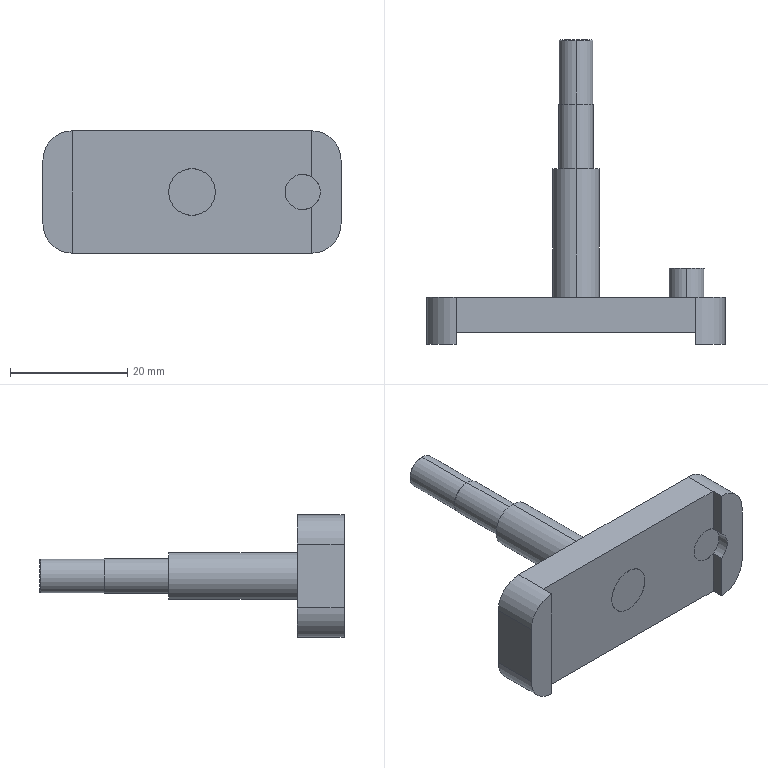Part | STEP file | BCC3 H14_9 | 3 solids | 35 faces | box 50.9 x 52 x 20.9 mm | volume 8450 mm3 | plane 17 | cylinder 16 | cone 2 | commonest cylinder face diameters 6 x6 10 x4 5.8 x2 7.95 x2 8 x2